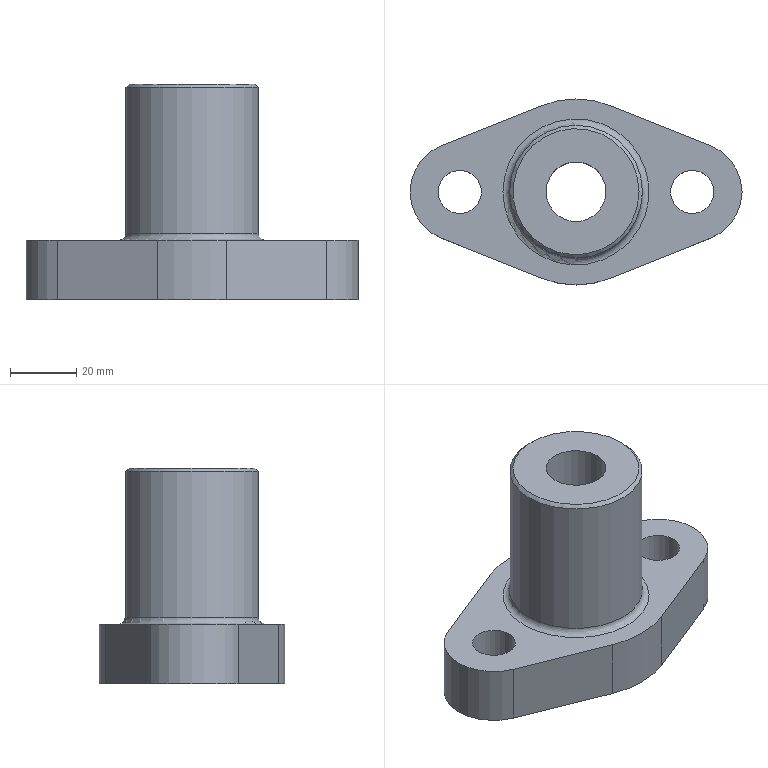Part | NX | features EXTRUDE 4, DATUM_CSYS 2, BLEND 1, CHAMFER 1, HOLE PACKAGE 1, SIMPLE HOLE 1, SKETCH 1, SYMBOLIC_THREAD 1 | 1 solid | 20 faces | box 100 x 56 x 65 mm | volume 108287 mm3 | cylinder 9 | plane 7 | cone 3 | torus 1 | commonest cylinder face diameters 13 x2 30 x2 56 x2 18 x1 18.5 x1 40 x1
STEP:
#1=CARTESIAN_POINT('',(40.571,-13.927,0.));
#2=VERTEX_POINT('',#1);
#3=CARTESIAN_POINT('',(10.4,-25.997,0.));
#4=VERTEX_POINT('',#3);
#5=CARTESIAN_POINT('',(40.571,-13.927,0.));
#6=DIRECTION('',(-0.9285,-0.3714,0.));
#7=VECTOR('',#6,1000.);
#8=LINE('',#5,#7);
#9=EDGE_CURVE('',#2,#4,#8,.T.);
#10=ORIENTED_EDGE('',*,*,#9,.F.);
#11=CARTESIAN_POINT('',(40.571,-13.927,18.));
#12=VERTEX_POINT('',#11);
#13=CARTESIAN_POINT('',(40.571,-13.927,18.));
#14=DIRECTION('',(0.,0.,-1.));
#15=VECTOR('',#14,1000.);
#16=LINE('',#13,#15);
#17=EDGE_CURVE('',#12,#2,#16,.T.);
#18=ORIENTED_EDGE('',*,*,#17,.F.);
#19=CARTESIAN_POINT('',(10.4,-25.997,18.));
#20=VERTEX_POINT('',#19);
#21=CARTESIAN_POINT('',(40.571,-13.927,18.));
#22=DIRECTION('',(-0.9285,-0.3714,0.));
#23=VECTOR('',#22,1000.);
#24=LINE('',#21,#23);
#25=EDGE_CURVE('',#12,#20,#24,.T.);
#26=ORIENTED_EDGE('',*,*,#25,.T.);
#27=CARTESIAN_POINT('',(10.4,-25.997,18.));
#28=DIRECTION('',(0.,0.,-1.));
#29=VECTOR('',#28,1000.);
#30=LINE('',#27,#29);
#31=EDGE_CURVE('',#20,#4,#30,.T.);
#32=ORIENTED_EDGE('',*,*,#31,.T.);
#33=EDGE_LOOP('',(#10,#18,#26,#32));
#34=FACE_BOUND('',#33,.T.);
#35=CARTESIAN_POINT('',(40.571,-13.927,18.));
#36=DIRECTION('',(0.3714,-0.9285,0.));
#37=DIRECTION('',(0.9285,0.3714,0.));
#38=AXIS2_PLACEMENT_3D('',#35,#36,#37);
#39=PLANE('',#38);
#40=ADVANCED_FACE('',(#34),#39,.T.);
#41=CARTESIAN_POINT('',(-10.4,-25.997,0.));
#42=VERTEX_POINT('',#41);
#43=CARTESIAN_POINT('',(0.,0.,0.));
#44=DIRECTION('',(0.,0.,-1.));
#45=DIRECTION('',(1.,0.,0.));
#46=AXIS2_PLACEMENT_3D('',#43,#44,#45);
#47=CIRCLE('',#46,28.);
#48=EDGE_CURVE('',#4,#42,#47,.T.);
#49=ORIENTED_EDGE('',*,*,#48,.F.);
#50=ORIENTED_EDGE('',*,*,#31,.F.);
#51=CARTESIAN_POINT('',(-10.4,-25.997,18.));
#52=VERTEX_POINT('',#51);
#53=CARTESIAN_POINT('',(0.,0.,18.));
#54=DIRECTION('',(0.,0.,-1.));
#55=DIRECTION('',(1.,0.,0.));
#56=AXIS2_PLACEMENT_3D('',#53,#54,#55);
#57=CIRCLE('',#56,28.);
#58=EDGE_CURVE('',#20,#52,#57,.T.);
#59=ORIENTED_EDGE('',*,*,#58,.T.);
#60=CARTESIAN_POINT('',(-10.4,-25.997,18.));
#61=DIRECTION('',(0.,0.,-1.));
#62=VECTOR('',#61,1000.);
#63=LINE('',#60,#62);
#64=EDGE_CURVE('',#52,#42,#63,.T.);
#65=ORIENTED_EDGE('',*,*,#64,.T.);
#66=EDGE_LOOP('',(#49,#50,#59,#65));
#67=FACE_BOUND('',#66,.T.);
#68=CARTESIAN_POINT('',(0.,0.,18.));
#69=DIRECTION('',(0.,0.,-1.));
#70=DIRECTION('',(-1.,0.,0.));
#71=AXIS2_PLACEMENT_3D('',#68,#69,#70);
#72=CYLINDRICAL_SURFACE('',#71,28.);
#73=ADVANCED_FACE('',(#67),#72,.T.);
#74=CARTESIAN_POINT('',(-40.571,-13.927,0.));
#75=VERTEX_POINT('',#74);
#76=CARTESIAN_POINT('',(-10.4,-25.997,0.));
#77=DIRECTION('',(-0.9285,0.3714,0.));
#78=VECTOR('',#77,1000.);
#79=LINE('',#76,#78);
#80=EDGE_CURVE('',#42,#75,#79,.T.);
#81=ORIENTED_EDGE('',*,*,#80,.F.);
#82=ORIENTED_EDGE('',*,*,#64,.F.);
#83=CARTESIAN_POINT('',(-40.571,-13.927,18.));
#84=VERTEX_POINT('',#83);
#85=CARTESIAN_POINT('',(-10.4,-25.997,18.));
#86=DIRECTION('',(-0.9285,0.3714,0.));
#87=VECTOR('',#86,1000.);
#88=LINE('',#85,#87);
#89=EDGE_CURVE('',#52,#84,#88,.T.);
#90=ORIENTED_EDGE('',*,*,#89,.T.);
#91=CARTESIAN_POINT('',(-40.571,-13.927,18.));
#92=DIRECTION('',(0.,0.,-1.));
#93=VECTOR('',#92,1000.);
#94=LINE('',#91,#93);
#95=EDGE_CURVE('',#84,#75,#94,.T.);
#96=ORIENTED_EDGE('',*,*,#95,.T.);
#97=EDGE_LOOP('',(#81,#82,#90,#96));
#98=FACE_BOUND('',#97,.T.);
#99=CARTESIAN_POINT('',(-10.4,-25.997,18.));
#100=DIRECTION('',(-0.3714,-0.9285,0.));
#101=DIRECTION('',(0.9285,-0.3714,0.));
#102=AXIS2_PLACEMENT_3D('',#99,#100,#101);
#103=PLANE('',#102);
#104=ADVANCED_FACE('',(#98),#103,.T.);
#105=CARTESIAN_POINT('',(-40.571,13.927,0.));
#106=VERTEX_POINT('',#105);
#107=CARTESIAN_POINT('',(-35.,0.,0.));
#108=DIRECTION('',(0.,0.,-1.));
#109=DIRECTION('',(1.,0.,0.));
#110=AXIS2_PLACEMENT_3D('',#107,#108,#109);
#111=CIRCLE('',#110,15.);
#112=EDGE_CURVE('',#75,#106,#111,.T.);
#113=ORIENTED_EDGE('',*,*,#112,.F.);
#114=ORIENTED_EDGE('',*,*,#95,.F.);
#115=CARTESIAN_POINT('',(-40.571,13.927,18.));
#116=VERTEX_POINT('',#115);
#117=CARTESIAN_POINT('',(-35.,0.,18.));
#118=DIRECTION('',(0.,0.,-1.));
#119=DIRECTION('',(1.,0.,0.));
#120=AXIS2_PLACEMENT_3D('',#117,#118,#119);
#121=CIRCLE('',#120,15.);
#122=EDGE_CURVE('',#84,#116,#121,.T.);
#123=ORIENTED_EDGE('',*,*,#122,.T.);
#124=CARTESIAN_POINT('',(-40.571,13.927,18.));
#125=DIRECTION('',(0.,0.,-1.));
#126=VECTOR('',#125,1000.);
#127=LINE('',#124,#126);
#128=EDGE_CURVE('',#116,#106,#127,.T.);
#129=ORIENTED_EDGE('',*,*,#128,.T.);
#130=EDGE_LOOP('',(#113,#114,#123,#129));
#131=FACE_BOUND('',#130,.T.);
#132=CARTESIAN_POINT('',(-35.,0.,18.));
#133=DIRECTION('',(0.,0.,-1.));
#134=DIRECTION('',(-1.,0.,0.));
#135=AXIS2_PLACEMENT_3D('',#132,#133,#134);
#136=CYLINDRICAL_SURFACE('',#135,15.);
#137=ADVANCED_FACE('',(#131),#136,.T.);
#138=CARTESIAN_POINT('',(-10.4,25.997,0.));
#139=VERTEX_POINT('',#138);
#140=CARTESIAN_POINT('',(-40.571,13.927,0.));
#141=DIRECTION('',(0.9285,0.3714,0.));
#142=VECTOR('',#141,1000.);
#143=LINE('',#140,#142);
#144=EDGE_CURVE('',#106,#139,#143,.T.);
#145=ORIENTED_EDGE('',*,*,#144,.F.);
#146=ORIENTED_EDGE('',*,*,#128,.F.);
#147=CARTESIAN_POINT('',(-10.4,25.997,18.));
#148=VERTEX_POINT('',#147);
#149=CARTESIAN_POINT('',(-40.571,13.927,18.));
#150=DIRECTION('',(0.9285,0.3714,0.));
#151=VECTOR('',#150,1000.);
#152=LINE('',#149,#151);
#153=EDGE_CURVE('',#116,#148,#152,.T.);
#154=ORIENTED_EDGE('',*,*,#153,.T.);
#155=CARTESIAN_POINT('',(-10.4,25.997,18.));
#156=DIRECTION('',(0.,0.,-1.));
#157=VECTOR('',#156,1000.);
#158=LINE('',#155,#157);
#159=EDGE_CURVE('',#148,#139,#158,.T.);
#160=ORIENTED_EDGE('',*,*,#159,.T.);
#161=EDGE_LOOP('',(#145,#146,#154,#160));
#162=FACE_BOUND('',#161,.T.);
#163=CARTESIAN_POINT('',(-40.571,13.927,18.));
#164=DIRECTION('',(-0.3714,0.9285,0.));
#165=DIRECTION('',(-0.9285,-0.3714,0.));
#166=AXIS2_PLACEMENT_3D('',#163,#164,#165);
#167=PLANE('',#166);
#168=ADVANCED_FACE('',(#162),#167,.T.);
#169=CARTESIAN_POINT('',(10.4,25.997,0.));
#170=VERTEX_POINT('',#169);
#171=CARTESIAN_POINT('',(0.,0.,0.));
#172=DIRECTION('',(0.,0.,-1.));
#173=DIRECTION('',(1.,0.,0.));
#174=AXIS2_PLACEMENT_3D('',#171,#172,#173);
#175=CIRCLE('',#174,28.);
#176=EDGE_CURVE('',#139,#170,#175,.T.);
#177=ORIENTED_EDGE('',*,*,#176,.F.);
#178=ORIENTED_EDGE('',*,*,#159,.F.);
#179=CARTESIAN_POINT('',(10.4,25.997,18.));
#180=VERTEX_POINT('',#179);
#181=CARTESIAN_POINT('',(0.,0.,18.));
#182=DIRECTION('',(0.,0.,-1.));
#183=DIRECTION('',(1.,0.,0.));
#184=AXIS2_PLACEMENT_3D('',#181,#182,#183);
#185=CIRCLE('',#184,28.);
#186=EDGE_CURVE('',#148,#180,#185,.T.);
#187=ORIENTED_EDGE('',*,*,#186,.T.);
#188=CARTESIAN_POINT('',(10.4,25.997,18.));
#189=DIRECTION('',(0.,0.,-1.));
#190=VECTOR('',#189,1000.);
#191=LINE('',#188,#190);
#192=EDGE_CURVE('',#180,#170,#191,.T.);
#193=ORIENTED_EDGE('',*,*,#192,.T.);
#194=EDGE_LOOP('',(#177,#178,#187,#193));
#195=FACE_BOUND('',#194,.T.);
#196=CARTESIAN_POINT('',(0.,0.,18.));
#197=DIRECTION('',(0.,0.,-1.));
#198=DIRECTION('',(-1.,0.,0.));
#199=AXIS2_PLACEMENT_3D('',#196,#197,#198);
#200=CYLINDRICAL_SURFACE('',#199,28.);
#201=ADVANCED_FACE('',(#195),#200,.T.);
#202=CARTESIAN_POINT('',(40.571,13.927,0.));
#203=VERTEX_POINT('',#202);
#204=CARTESIAN_POINT('',(10.4,25.997,0.));
#205=DIRECTION('',(0.9285,-0.3714,0.));
#206=VECTOR('',#205,1000.);
#207=LINE('',#204,#206);
#208=EDGE_CURVE('',#170,#203,#207,.T.);
#209=ORIENTED_EDGE('',*,*,#208,.F.);
#210=ORIENTED_EDGE('',*,*,#192,.F.);
#211=CARTESIAN_POINT('',(40.571,13.927,18.));
#212=VERTEX_POINT('',#211);
#213=CARTESIAN_POINT('',(10.4,25.997,18.));
#214=DIRECTION('',(0.9285,-0.3714,0.));
#215=VECTOR('',#214,1000.);
#216=LINE('',#213,#215);
#217=EDGE_CURVE('',#180,#212,#216,.T.);
#218=ORIENTED_EDGE('',*,*,#217,.T.);
#219=CARTESIAN_POINT('',(40.571,13.927,18.));
#220=DIRECTION('',(0.,0.,-1.));
#221=VECTOR('',#220,1000.);
#222=LINE('',#219,#221);
#223=EDGE_CURVE('',#212,#203,#222,.T.);
#224=ORIENTED_EDGE('',*,*,#223,.T.);
#225=EDGE_LOOP('',(#209,#210,#218,#224));
#226=FACE_BOUND('',#225,.T.);
#227=CARTESIAN_POINT('',(10.4,25.997,18.));
#228=DIRECTION('',(0.3714,0.9285,0.));
#229=DIRECTION('',(-0.9285,0.3714,0.));
#230=AXIS2_PLACEMENT_3D('',#227,#228,#229);
#231=PLANE('',#230);
#232=ADVANCED_FACE('',(#226),#231,.T.);
#233=CARTESIAN_POINT('',(35.,0.,0.));
#234=DIRECTION('',(0.,0.,-1.));
#235=DIRECTION('',(1.,0.,0.));
#236=AXIS2_PLACEMENT_3D('',#233,#234,#235);
#237=CIRCLE('',#236,15.);
#238=EDGE_CURVE('',#203,#2,#237,.T.);
#239=ORIENTED_EDGE('',*,*,#238,.F.);
#240=ORIENTED_EDGE('',*,*,#223,.F.);
#241=CARTESIAN_POINT('',(35.,0.,18.));
#242=DIRECTION('',(0.,0.,-1.));
#243=DIRECTION('',(1.,0.,0.));
#244=AXIS2_PLACEMENT_3D('',#241,#242,#243);
#245=CIRCLE('',#244,15.);
#246=EDGE_CURVE('',#212,#12,#245,.T.);
#247=ORIENTED_EDGE('',*,*,#246,.T.);
#248=ORIENTED_EDGE('',*,*,#17,.T.);
#249=EDGE_LOOP('',(#239,#240,#247,#248));
#250=FACE_BOUND('',#249,.T.);
#251=CARTESIAN_POINT('',(35.,0.,18.));
#252=DIRECTION('',(0.,0.,-1.));
#253=DIRECTION('',(-1.,0.,0.));
#254=AXIS2_PLACEMENT_3D('',#251,#252,#253);
#255=CYLINDRICAL_SURFACE('',#254,15.);
#256=ADVANCED_FACE('',(#250),#255,.T.);
#257=CARTESIAN_POINT('',(-22.,0.,18.));
#258=VERTEX_POINT('',#257);
#259=CARTESIAN_POINT('',(0.,0.,18.));
#260=DIRECTION('',(0.,0.,-1.));
#261=DIRECTION('',(-1.,0.,0.));
#262=AXIS2_PLACEMENT_3D('',#259,#260,#261);
#263=CIRCLE('',#262,22.);
#264=EDGE_CURVE('',#258,#258,#263,.T.);
#265=ORIENTED_EDGE('',*,*,#264,.T.);
#266=EDGE_LOOP('',(#265));
#267=FACE_BOUND('',#266,.T.);
#268=CARTESIAN_POINT('',(-41.5,0.,18.));
#269=VERTEX_POINT('',#268);
#270=CARTESIAN_POINT('',(-35.,0.,18.));
#271=DIRECTION('',(0.,0.,-1.));
#272=DIRECTION('',(-1.,0.,0.));
#273=AXIS2_PLACEMENT_3D('',#270,#271,#272);
#274=CIRCLE('',#273,6.5);
#275=EDGE_CURVE('',#269,#269,#274,.F.);
#276=ORIENTED_EDGE('',*,*,#275,.F.);
#277=EDGE_LOOP('',(#276));
#278=FACE_BOUND('',#277,.T.);
#279=CARTESIAN_POINT('',(28.5,0.,18.));
#280=VERTEX_POINT('',#279);
#281=CARTESIAN_POINT('',(35.,0.,18.));
#282=DIRECTION('',(0.,0.,-1.));
#283=DIRECTION('',(-1.,0.,0.));
#284=AXIS2_PLACEMENT_3D('',#281,#282,#283);
#285=CIRCLE('',#284,6.5);
#286=EDGE_CURVE('',#280,#280,#285,.F.);
#287=ORIENTED_EDGE('',*,*,#286,.F.);
#288=EDGE_LOOP('',(#287));
#289=FACE_BOUND('',#288,.T.);
#290=ORIENTED_EDGE('',*,*,#25,.F.);
#291=ORIENTED_EDGE('',*,*,#246,.F.);
#292=ORIENTED_EDGE('',*,*,#217,.F.);
#293=ORIENTED_EDGE('',*,*,#186,.F.);
#294=ORIENTED_EDGE('',*,*,#153,.F.);
#295=ORIENTED_EDGE('',*,*,#122,.F.);
#296=ORIENTED_EDGE('',*,*,#89,.F.);
#297=ORIENTED_EDGE('',*,*,#58,.F.);
#298=EDGE_LOOP('',(#290,#291,#292,#293,#294,#295,#296,#297));
#299=FACE_BOUND('',#298,.T.);
#300=CARTESIAN_POINT('',(0.,0.,18.));
#301=DIRECTION('',(0.,0.,-1.));
#302=DIRECTION('',(-1.,0.,0.));
#303=AXIS2_PLACEMENT_3D('',#300,#301,#302);
#304=PLANE('',#303);
#305=ADVANCED_FACE('',(#267,#278,#289,#299),#304,.F.);
#306=CARTESIAN_POINT('',(-10.,0.,0.));
#307=VERTEX_POINT('',#306);
#308=CARTESIAN_POINT('',(0.,0.,0.));
#309=DIRECTION('',(0.,0.,-1.));
#310=DIRECTION('',(-1.,0.,0.));
#311=AXIS2_PLACEMENT_3D('',#308,#309,#310);
#312=CIRCLE('',#311,10.);
#313=EDGE_CURVE('',#307,#307,#312,.F.);
#314=ORIENTED_EDGE('',*,*,#313,.T.);
#315=EDGE_LOOP('',(#314));
#316=FACE_BOUND('',#315,.T.);
#317=CARTESIAN_POINT('',(-28.5,0.,0.));
#318=VERTEX_POINT('',#317);
#319=CARTESIAN_POINT('',(-35.,0.,0.));
#320=DIRECTION('',(0.,0.,1.));
#321=DIRECTION('',(1.,0.,0.));
#322=AXIS2_PLACEMENT_3D('',#319,#320,#321);
#323=CIRCLE('',#322,6.5);
#324=EDGE_CURVE('',#318,#318,#323,.T.);
#325=ORIENTED_EDGE('',*,*,#324,.T.);
#326=EDGE_LOOP('',(#325));
#327=FACE_BOUND('',#326,.T.);
#328=CARTESIAN_POINT('',(41.5,0.,0.));
#329=VERTEX_POINT('',#328);
#330=CARTESIAN_POINT('',(35.,0.,0.));
#331=DIRECTION('',(0.,0.,1.));
#332=DIRECTION('',(1.,0.,0.));
#333=AXIS2_PLACEMENT_3D('',#330,#331,#332);
#334=CIRCLE('',#333,6.5);
#335=EDGE_CURVE('',#329,#329,#334,.T.);
#336=ORIENTED_EDGE('',*,*,#335,.T.);
#337=EDGE_LOOP('',(#336));
#338=FACE_BOUND('',#337,.T.);
#339=ORIENTED_EDGE('',*,*,#9,.T.);
#340=ORIENTED_EDGE('',*,*,#48,.T.);
#341=ORIENTED_EDGE('',*,*,#80,.T.);
#342=ORIENTED_EDGE('',*,*,#112,.T.);
#343=ORIENTED_EDGE('',*,*,#144,.T.);
#344=ORIENTED_EDGE('',*,*,#176,.T.);
#345=ORIENTED_EDGE('',*,*,#208,.T.);
#346=ORIENTED_EDGE('',*,*,#238,.T.);
#347=EDGE_LOOP('',(#339,#340,#341,#342,#343,#344,#345,#346));
#348=FACE_BOUND('',#347,.T.);
#349=CARTESIAN_POINT('',(0.,0.,0.));
#350=DIRECTION('',(0.,0.,-1.));
#351=DIRECTION('',(-1.,0.,0.));
#352=AXIS2_PLACEMENT_3D('',#349,#350,#351);
#353=PLANE('',#352);
#354=ADVANCED_FACE('',(#316,#327,#338,#348),#353,.T.);
#355=CARTESIAN_POINT('',(20.,0.,64.));
#356=VERTEX_POINT('',#355);
#357=CARTESIAN_POINT('',(0.,0.,64.));
#358=DIRECTION('',(0.,0.,1.));
#359=DIRECTION('',(1.,0.,0.));
#360=AXIS2_PLACEMENT_3D('',#357,#358,#359);
#361=CIRCLE('',#360,20.);
#362=EDGE_CURVE('',#356,#356,#361,.F.);
#363=ORIENTED_EDGE('',*,*,#362,.T.);
#364=EDGE_LOOP('',(#363));
#365=FACE_BOUND('',#364,.T.);
#366=CARTESIAN_POINT('',(-20.,0.,20.));
#367=VERTEX_POINT('',#366);
#368=CARTESIAN_POINT('',(0.,0.,20.));
#369=DIRECTION('',(0.,0.,-1.));
#370=DIRECTION('',(-1.,0.,0.));
#371=AXIS2_PLACEMENT_3D('',#368,#369,#370);
#372=CIRCLE('',#371,20.);
#373=EDGE_CURVE('',#367,#367,#372,.F.);
#374=ORIENTED_EDGE('',*,*,#373,.T.);
#375=EDGE_LOOP('',(#374));
#376=FACE_BOUND('',#375,.T.);
#377=CARTESIAN_POINT('',(0.,0.,65.));
#378=DIRECTION('',(0.,0.,-1.));
#379=DIRECTION('',(-1.,0.,0.));
#380=AXIS2_PLACEMENT_3D('',#377,#378,#379);
#381=CYLINDRICAL_SURFACE('',#380,20.);
#382=ADVANCED_FACE('',(#365,#376),#381,.T.);
#383=CARTESIAN_POINT('',(19.,0.,65.));
#384=VERTEX_POINT('',#383);
#385=CARTESIAN_POINT('',(0.,0.,65.));
#386=DIRECTION('',(0.,0.,1.));
#387=DIRECTION('',(1.,0.,0.));
#388=AXIS2_PLACEMENT_3D('',#385,#386,#387);
#389=CIRCLE('',#388,19.);
#390=EDGE_CURVE('',#384,#384,#389,.T.);
#391=ORIENTED_EDGE('',*,*,#390,.T.);
#392=EDGE_LOOP('',(#391));
#393=FACE_BOUND('',#392,.T.);
#394=CARTESIAN_POINT('',(9.,0.,65.));
#395=VERTEX_POINT('',#394);
#396=CARTESIAN_POINT('',(0.,0.,65.));
#397=DIRECTION('',(0.,0.,-1.));
#398=DIRECTION('',(1.,0.,0.));
#399=AXIS2_PLACEMENT_3D('',#396,#397,#398);
#400=CIRCLE('',#399,9.);
#401=EDGE_CURVE('',#395,#395,#400,.T.);
#402=ORIENTED_EDGE('',*,*,#401,.T.);
#403=EDGE_LOOP('',(#402));
#404=FACE_BOUND('',#403,.T.);
#405=CARTESIAN_POINT('',(0.,0.,65.));
#406=DIRECTION('',(0.,0.,1.));
#407=DIRECTION('',(1.,0.,0.));
#408=AXIS2_PLACEMENT_3D('',#405,#406,#407);
#409=PLANE('',#408);
#410=ADVANCED_FACE('',(#393,#404),#409,.T.);
#411=ORIENTED_EDGE('',*,*,#335,.F.);
#412=EDGE_LOOP('',(#411));
#413=FACE_BOUND('',#412,.T.);
#414=ORIENTED_EDGE('',*,*,#286,.T.);
#415=EDGE_LOOP('',(#414));
#416=FACE_BOUND('',#415,.T.);
#417=CARTESIAN_POINT('',(35.,0.,65.));
#418=DIRECTION('',(0.,0.,-1.));
#419=DIRECTION('',(-1.,0.,0.));
#420=AXIS2_PLACEMENT_3D('',#417,#418,#419);
#421=CYLINDRICAL_SURFACE('',#420,6.5);
#422=ADVANCED_FACE('',(#413,#416),#421,.F.);
#423=ORIENTED_EDGE('',*,*,#324,.F.);
#424=EDGE_LOOP('',(#423));
#425=FACE_BOUND('',#424,.T.);
#426=ORIENTED_EDGE('',*,*,#275,.T.);
#427=EDGE_LOOP('',(#426));
#428=FACE_BOUND('',#427,.T.);
#429=CARTESIAN_POINT('',(-35.,0.,65.));
#430=DIRECTION('',(0.,0.,-1.));
#431=DIRECTION('',(-1.,0.,0.));
#432=AXIS2_PLACEMENT_3D('',#429,#430,#431);
#433=CYLINDRICAL_SURFACE('',#432,6.5);
#434=ADVANCED_FACE('',(#425,#428),#433,.F.);
#435=CARTESIAN_POINT('',(-9.,0.,12.15));
#436=VERTEX_POINT('',#435);
#437=CARTESIAN_POINT('',(0.,0.,12.15));
#438=DIRECTION('',(0.,0.,-1.));
#439=DIRECTION('',(-1.,0.,0.));
#440=AXIS2_PLACEMENT_3D('',#437,#438,#439);
#441=CIRCLE('',#440,9.);
#442=EDGE_CURVE('',#436,#436,#441,.F.);
#443=ORIENTED_EDGE('',*,*,#442,.T.);
#444=EDGE_LOOP('',(#443));
#445=FACE_BOUND('',#444,.T.);
#446=CARTESIAN_POINT('',(9.25,0.,12.));
#447=VERTEX_POINT('',#446);
#448=CARTESIAN_POINT('',(0.,0.,12.));
#449=DIRECTION('',(0.,0.,1.));
#450=DIRECTION('',(1.,0.,0.));
#451=AXIS2_PLACEMENT_3D('',#448,#449,#450);
#452=CIRCLE('',#451,9.25);
#453=EDGE_CURVE('',#447,#447,#452,.F.);
#454=ORIENTED_EDGE('',*,*,#453,.T.);
#455=EDGE_LOOP('',(#454));
#456=FACE_BOUND('',#455,.T.);
#457=CARTESIAN_POINT('',(0.,0.,12.));
#458=DIRECTION('',(0.,0.,-1.));
#459=DIRECTION('',(-1.,0.,0.));
#460=AXIS2_PLACEMENT_3D('',#457,#458,#459);
#461=CONICAL_SURFACE('',#460,9.25,1.03);
#462=ADVANCED_FACE('',(#445,#456),#461,.F.);
#463=CARTESIAN_POINT('',(-9.25,0.,0.75));
#464=VERTEX_POINT('',#463);
#465=CARTESIAN_POINT('',(0.,0.,0.75));
#466=DIRECTION('',(0.,0.,-1.));
#467=DIRECTION('',(-1.,0.,0.));
#468=AXIS2_PLACEMENT_3D('',#465,#466,#467);
#469=CIRCLE('',#468,9.25);
#470=EDGE_CURVE('',#464,#464,#469,.T.);
#471=ORIENTED_EDGE('',*,*,#470,.T.);
#472=EDGE_LOOP('',(#471));
#473=FACE_BOUND('',#472,.T.);
#474=ORIENTED_EDGE('',*,*,#453,.F.);
#475=EDGE_LOOP('',(#474));
#476=FACE_BOUND('',#475,.T.);
#477=CARTESIAN_POINT('',(0.,0.,0.));
#478=DIRECTION('',(0.,0.,1.));
#479=DIRECTION('',(1.,0.,0.));
#480=AXIS2_PLACEMENT_3D('',#477,#478,#479);
#481=CYLINDRICAL_SURFACE('',#480,9.25);
#482=ADVANCED_FACE('',(#473,#476),#481,.F.);
#483=ORIENTED_EDGE('',*,*,#470,.F.);
#484=EDGE_LOOP('',(#483));
#485=FACE_BOUND('',#484,.T.);
#486=ORIENTED_EDGE('',*,*,#313,.F.);
#487=EDGE_LOOP('',(#486));
#488=FACE_BOUND('',#487,.T.);
#489=CARTESIAN_POINT('',(0.,0.,0.));
#490=DIRECTION('',(0.,0.,-1.));
#491=DIRECTION('',(-1.,0.,0.));
#492=AXIS2_PLACEMENT_3D('',#489,#490,#491);
#493=CONICAL_SURFACE('',#492,10.,0.7854);
#494=ADVANCED_FACE('',(#485,#488),#493,.F.);
#495=ORIENTED_EDGE('',*,*,#401,.F.);
#496=EDGE_LOOP('',(#495));
#497=FACE_BOUND('',#496,.T.);
#498=ORIENTED_EDGE('',*,*,#442,.F.);
#499=EDGE_LOOP('',(#498));
#500=FACE_BOUND('',#499,.T.);
#501=CARTESIAN_POINT('',(0.,0.,65.));
#502=DIRECTION('',(0.,0.,-1.));
#503=DIRECTION('',(-1.,0.,0.));
#504=AXIS2_PLACEMENT_3D('',#501,#502,#503);
#505=CYLINDRICAL_SURFACE('',#504,9.);
#506=ADVANCED_FACE('',(#497,#500),#505,.F.);
#507=ORIENTED_EDGE('',*,*,#264,.F.);
#508=EDGE_LOOP('',(#507));
#509=FACE_BOUND('',#508,.T.);
#510=ORIENTED_EDGE('',*,*,#373,.F.);
#511=EDGE_LOOP('',(#510));
#512=FACE_BOUND('',#511,.T.);
#513=CARTESIAN_POINT('',(0.,0.,20.));
#514=DIRECTION('',(0.,0.,-1.));
#515=DIRECTION('',(-1.,0.,0.));
#516=AXIS2_PLACEMENT_3D('',#513,#514,#515);
#517=TOROIDAL_SURFACE('',#516,22.,2.);
#518=ADVANCED_FACE('',(#509,#512),#517,.F.);
#519=ORIENTED_EDGE('',*,*,#362,.F.);
#520=EDGE_LOOP('',(#519));
#521=FACE_BOUND('',#520,.T.);
#522=ORIENTED_EDGE('',*,*,#390,.F.);
#523=EDGE_LOOP('',(#522));
#524=FACE_BOUND('',#523,.T.);
#525=CARTESIAN_POINT('',(0.,0.,65.));
#526=DIRECTION('',(0.,0.,-1.));
#527=DIRECTION('',(-1.,0.,0.));
#528=AXIS2_PLACEMENT_3D('',#525,#526,#527);
#529=CONICAL_SURFACE('',#528,19.,0.7854);
#530=ADVANCED_FACE('',(#521,#524),#529,.T.);
#531=CLOSED_SHELL('',(#40,#73,#104,#137,#168,#201,#232,#256,#305,#354,#382,#410,#422,#434,#462,#482,#494,#506,#518,#530));
#532=MANIFOLD_SOLID_BREP('',#531);
#533=(LENGTH_UNIT()NAMED_UNIT(*)SI_UNIT(.MILLI.,.METRE.));
#534=UNCERTAINTY_MEASURE_WITH_UNIT(LENGTH_MEASURE(0.00001),#533,'','');
#535=(NAMED_UNIT(*)PLANE_ANGLE_UNIT()SI_UNIT($,.RADIAN.));
#536=(NAMED_UNIT(*)SI_UNIT($,.STERADIAN.)SOLID_ANGLE_UNIT());
#537=(GEOMETRIC_REPRESENTATION_CONTEXT(3)GLOBAL_UNCERTAINTY_ASSIGNED_CONTEXT((#534))GLOBAL_UNIT_ASSIGNED_CONTEXT((#533,#535,#536))REPRESENTATION_CONTEXT('',''));
#538=ADVANCED_BREP_SHAPE_REPRESENTATION('',(#532),#537);